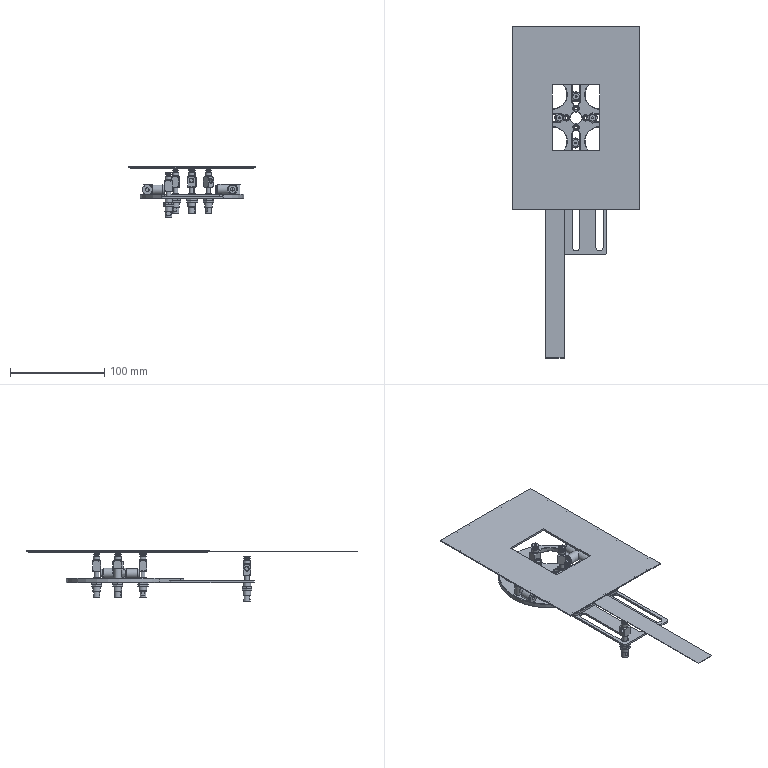Part | NX | 6 solids | 632 faces | box 135 x 352.5 x 54.5 mm | volume 99869 mm3 | plane 252 | cone 241 | cylinder 113 | torus 25 | spline 1 | commonest cylinder face diameters 7 x28 8.2 x14 4 x11 8 x7 2.5 x6 10.4 x6